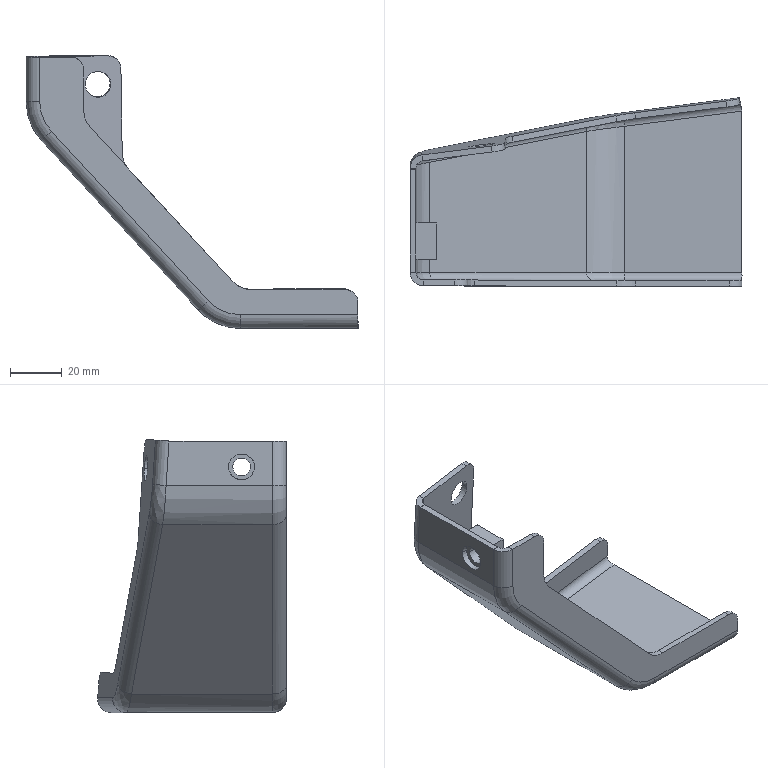Part | SolidWorks | features MBimport 1 | 2 solids | 71 faces | box 128.4 x 72.927 x 105.583 mm | volume 38422 mm3 | plane 31 | cylinder 30 | spline 6 | torus 4 | commonest cylinder face diameters 10 x8 6 x6 10.6 x6 20 x4 6.75 x2 40 x2